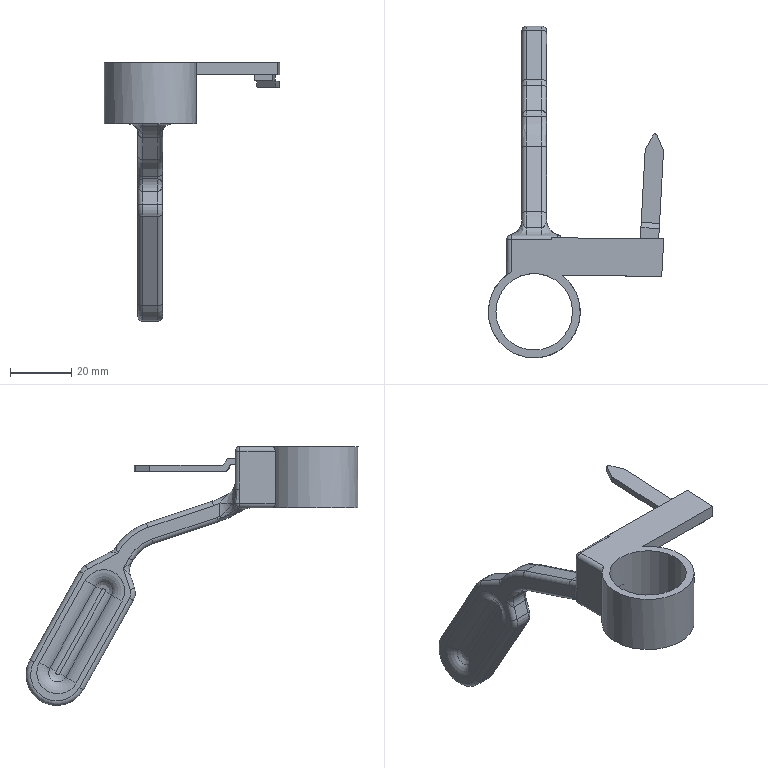Part | STEP file | DEWALT-DWE7492-B22 | 1 solid | 122 faces | box 57.196 x 108.227 x 84.374 mm | volume 18849 mm3 | cylinder 46 | plane 34 | torus 20 | spline 14 | sphere 4 | other 4 | commonest cylinder face diameters 3 x22 10 x12 6 x4 1.4 x1 20 x1 23.71 x1